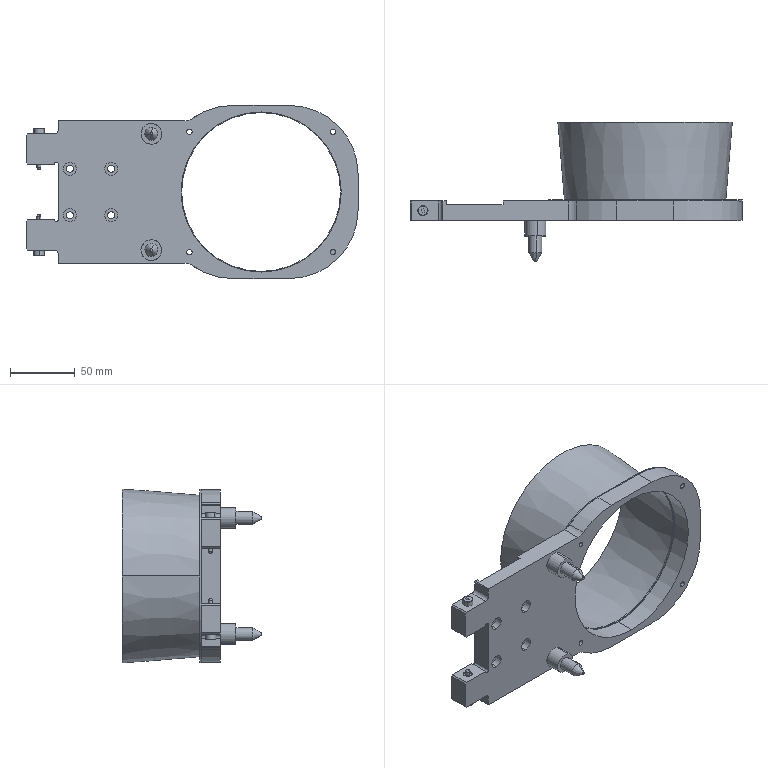Part | SolidWorks | 8 solids | 202 faces | box 257 x 108 x 135 mm | volume 263904 mm3 | cylinder 91 | plane 81 | cone 26 | sphere 4 | commonest cylinder face diameters 5.5 x20 10 x16 4.2 x12 16 x8 106 x8 3.1 x4